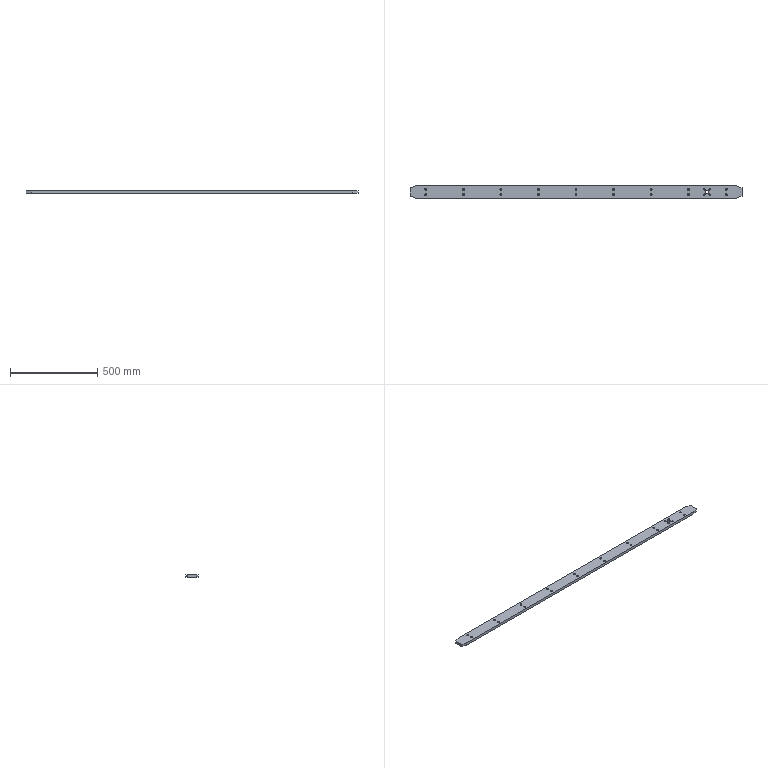Part | STEP file | Nylon backrest plate 1 | 1 solid | 110 faces | box 1900 x 69 x 16 mm | volume 2062797 mm3 | cylinder 82 | plane 28 | commonest cylinder face diameters 6.4 x36 11 x36 8 x8 20 x2